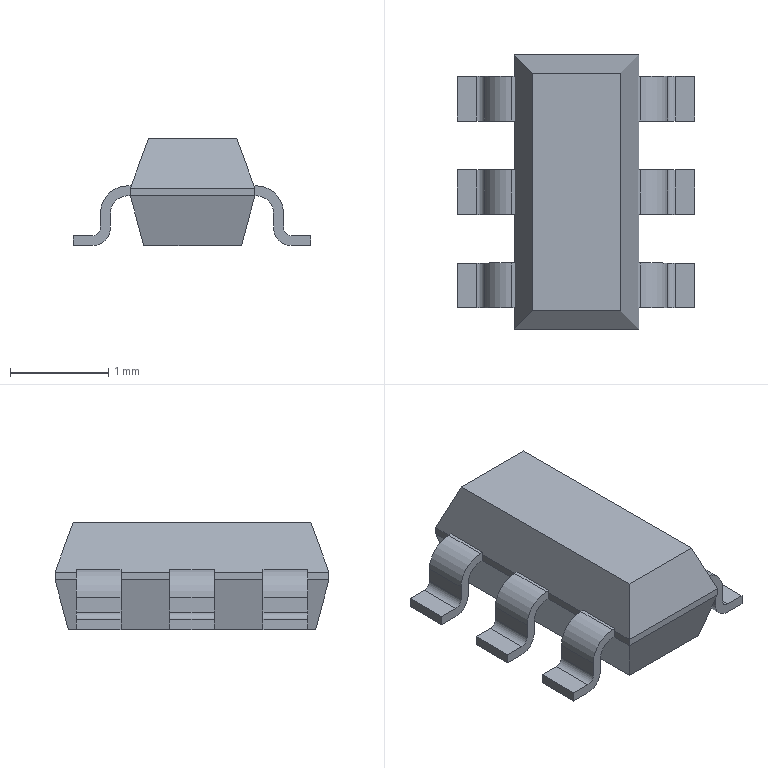Part | STEP file | RJ-USIO-V1_2-220411_192 | 1 solid | 98 faces | box 2.426 x 2.794 x 1.092 mm | volume 3.509 mm3 | plane 74 | cylinder 24 | commonest cylinder face diameters 0.356 x12 0.152 x6 0.559 x6